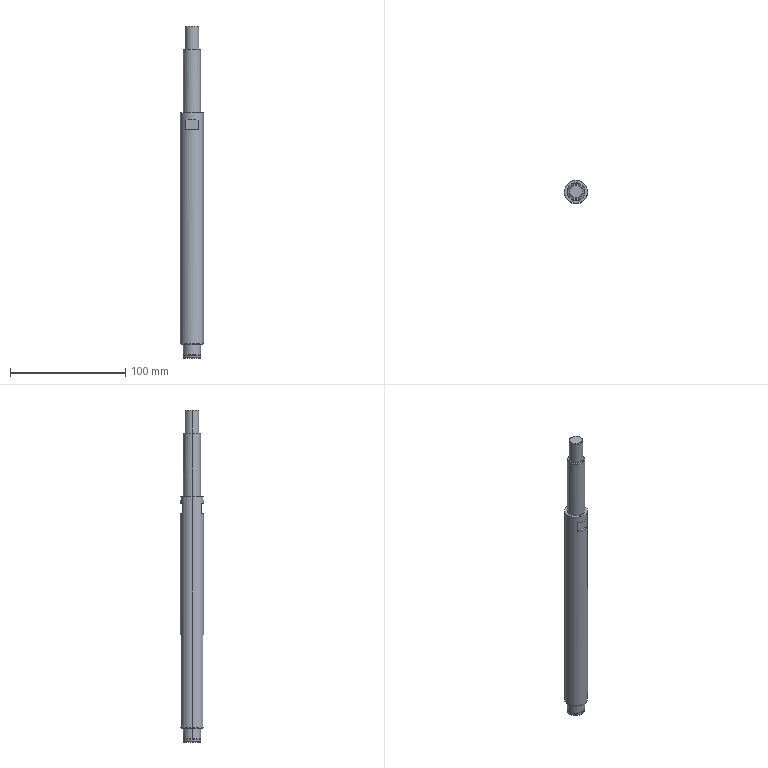Part | SolidWorks | features BaseBody 1 | 1 solid | 37 faces | box 20 x 20 x 287.5 mm | volume 76758 mm3 | plane 13 | cylinder 12 | cone 8 | spline 4 | commonest cylinder face diameters 15 x6 12 x2 14.3 x2 20 x2
STEP:
#1=CARTESIAN_POINT('',(-127.496,1839.044,-21.2));
#2=VERTEX_POINT('',#1);
#3=CARTESIAN_POINT('',(-134.996,1831.544,-21.2));
#4=VERTEX_POINT('',#3);
#5=CARTESIAN_POINT('',(-127.496,1831.544,-21.2));
#6=DIRECTION('',(0.,0.,1.));
#7=DIRECTION('',(0.,-1.,0.));
#8=AXIS2_PLACEMENT_3D('',#5,#6,#7);
#9=CIRCLE('',#8,7.5);
#10=EDGE_CURVE('',#2,#4,#9,.T.);
#11=ORIENTED_EDGE('',*,*,#10,.F.);
#12=CARTESIAN_POINT('',(-127.496,1839.344,-21.5));
#13=VERTEX_POINT('',#12);
#14=CARTESIAN_POINT('',(-127.496,1839.344,-21.2));
#15=DIRECTION('',(1.,0.,0.));
#16=DIRECTION('',(0.,1.,0.));
#17=AXIS2_PLACEMENT_3D('',#14,#15,#16);
#18=CIRCLE('',#17,0.3);
#19=EDGE_CURVE('',#2,#13,#18,.T.);
#20=ORIENTED_EDGE('',*,*,#19,.T.);
#21=CARTESIAN_POINT('',(-127.496,1823.744,-21.5));
#22=VERTEX_POINT('',#21);
#23=CARTESIAN_POINT('',(-127.496,1839.344,-21.5));
#24=CARTESIAN_POINT('',(-143.096,1839.344,-21.5));
#25=CARTESIAN_POINT('',(-143.096,1823.744,-21.5));
#26=CARTESIAN_POINT('',(-127.496,1823.744,-21.5));
#27=(BOUNDED_CURVE()B_SPLINE_CURVE(3,(#23,#24,#25,#26),.UNSPECIFIED.,.F.,.F.)B_SPLINE_CURVE_WITH_KNOTS((4,4),(0.,1.),.UNSPECIFIED.)CURVE()GEOMETRIC_REPRESENTATION_ITEM()RATIONAL_B_SPLINE_CURVE((1.,0.3333,0.3333,1.))REPRESENTATION_ITEM(''));
#28=EDGE_CURVE('',#13,#22,#27,.T.);
#29=ORIENTED_EDGE('',*,*,#28,.T.);
#30=CARTESIAN_POINT('',(-127.496,1824.044,-21.2));
#31=VERTEX_POINT('',#30);
#32=CARTESIAN_POINT('',(-127.496,1823.744,-21.2));
#33=DIRECTION('',(-1.,0.,0.));
#34=DIRECTION('',(0.,-1.,0.));
#35=AXIS2_PLACEMENT_3D('',#32,#33,#34);
#36=CIRCLE('',#35,0.3);
#37=EDGE_CURVE('',#31,#22,#36,.T.);
#38=ORIENTED_EDGE('',*,*,#37,.F.);
#39=CARTESIAN_POINT('',(-127.496,1831.544,-21.2));
#40=DIRECTION('',(0.,0.,1.));
#41=DIRECTION('',(0.,-1.,0.));
#42=AXIS2_PLACEMENT_3D('',#39,#40,#41);
#43=CIRCLE('',#42,7.5);
#44=EDGE_CURVE('',#4,#31,#43,.T.);
#45=ORIENTED_EDGE('',*,*,#44,.F.);
#46=EDGE_LOOP('',(#11,#20,#29,#38,#45));
#47=FACE_OUTER_BOUND('',#46,.T.);
#48=CARTESIAN_POINT('',(-127.496,1824.044,-21.2));
#49=CARTESIAN_POINT('',(-142.496,1824.044,-21.2));
#50=CARTESIAN_POINT('',(-142.496,1839.044,-21.2));
#51=CARTESIAN_POINT('',(-127.496,1839.044,-21.2));
#52=CARTESIAN_POINT('',(-127.496,1824.044,-21.376));
#53=CARTESIAN_POINT('',(-142.496,1824.044,-21.376));
#54=CARTESIAN_POINT('',(-142.496,1839.044,-21.376));
#55=CARTESIAN_POINT('',(-127.496,1839.044,-21.376));
#56=CARTESIAN_POINT('',(-127.496,1823.92,-21.5));
#57=CARTESIAN_POINT('',(-142.744,1823.92,-21.5));
#58=CARTESIAN_POINT('',(-142.744,1839.168,-21.5));
#59=CARTESIAN_POINT('',(-127.496,1839.168,-21.5));
#60=CARTESIAN_POINT('',(-127.496,1823.744,-21.5));
#61=CARTESIAN_POINT('',(-143.096,1823.744,-21.5));
#62=CARTESIAN_POINT('',(-143.096,1839.344,-21.5));
#63=CARTESIAN_POINT('',(-127.496,1839.344,-21.5));
#64=(BOUNDED_SURFACE()B_SPLINE_SURFACE(3,3,((#48,#49,#50,#51),(#52,#53,#54,#55),(#56,#57,#58,#59),(#60,#61,#62,#63)),.UNSPECIFIED.,.F.,.F.,.T.)B_SPLINE_SURFACE_WITH_KNOTS((4,4),(4,4),(0.,1.),(0.,1.),.UNSPECIFIED.)GEOMETRIC_REPRESENTATION_ITEM()RATIONAL_B_SPLINE_SURFACE(((1.,0.3333,0.3333,1.),(0.8047,0.2682,0.2682,0.8047),(0.8047,0.2682,0.2682,0.8047),(1.,0.3333,0.3333,1.)))REPRESENTATION_ITEM('')SURFACE());
#65=ADVANCED_FACE('',(#47),#64,.F.);
#66=CARTESIAN_POINT('',(-127.496,1824.044,-222.3));
#67=VERTEX_POINT('',#66);
#68=CARTESIAN_POINT('',(-134.996,1831.544,-222.3));
#69=VERTEX_POINT('',#68);
#70=CARTESIAN_POINT('',(-127.496,1831.544,-222.3));
#71=DIRECTION('',(0.,0.,-1.));
#72=DIRECTION('',(0.,1.,0.));
#73=AXIS2_PLACEMENT_3D('',#70,#71,#72);
#74=CIRCLE('',#73,7.5);
#75=EDGE_CURVE('',#67,#69,#74,.T.);
#76=ORIENTED_EDGE('',*,*,#75,.F.);
#77=CARTESIAN_POINT('',(-127.496,1823.744,-222.));
#78=VERTEX_POINT('',#77);
#79=CARTESIAN_POINT('',(-127.496,1823.744,-222.3));
#80=DIRECTION('',(1.,0.,0.));
#81=DIRECTION('',(0.,-1.,0.));
#82=AXIS2_PLACEMENT_3D('',#79,#80,#81);
#83=CIRCLE('',#82,0.3);
#84=EDGE_CURVE('',#67,#78,#83,.T.);
#85=ORIENTED_EDGE('',*,*,#84,.T.);
#86=CARTESIAN_POINT('',(-127.496,1839.344,-222.));
#87=VERTEX_POINT('',#86);
#88=CARTESIAN_POINT('',(-127.496,1823.744,-222.));
#89=CARTESIAN_POINT('',(-143.096,1823.744,-222.));
#90=CARTESIAN_POINT('',(-143.096,1839.344,-222.));
#91=CARTESIAN_POINT('',(-127.496,1839.344,-222.));
#92=(BOUNDED_CURVE()B_SPLINE_CURVE(3,(#88,#89,#90,#91),.UNSPECIFIED.,.F.,.F.)B_SPLINE_CURVE_WITH_KNOTS((4,4),(0.,1.),.UNSPECIFIED.)CURVE()GEOMETRIC_REPRESENTATION_ITEM()RATIONAL_B_SPLINE_CURVE((1.,0.3333,0.3333,1.))REPRESENTATION_ITEM(''));
#93=EDGE_CURVE('',#78,#87,#92,.T.);
#94=ORIENTED_EDGE('',*,*,#93,.T.);
#95=CARTESIAN_POINT('',(-127.496,1839.044,-222.3));
#96=VERTEX_POINT('',#95);
#97=CARTESIAN_POINT('',(-127.496,1839.344,-222.3));
#98=DIRECTION('',(-1.,0.,0.));
#99=DIRECTION('',(0.,1.,0.));
#100=AXIS2_PLACEMENT_3D('',#97,#98,#99);
#101=CIRCLE('',#100,0.3);
#102=EDGE_CURVE('',#96,#87,#101,.T.);
#103=ORIENTED_EDGE('',*,*,#102,.F.);
#104=CARTESIAN_POINT('',(-127.496,1831.544,-222.3));
#105=DIRECTION('',(0.,0.,-1.));
#106=DIRECTION('',(0.,1.,0.));
#107=AXIS2_PLACEMENT_3D('',#104,#105,#106);
#108=CIRCLE('',#107,7.5);
#109=EDGE_CURVE('',#69,#96,#108,.T.);
#110=ORIENTED_EDGE('',*,*,#109,.F.);
#111=EDGE_LOOP('',(#76,#85,#94,#103,#110));
#112=FACE_OUTER_BOUND('',#111,.T.);
#113=CARTESIAN_POINT('',(-127.496,1839.044,-222.3));
#114=CARTESIAN_POINT('',(-142.496,1839.044,-222.3));
#115=CARTESIAN_POINT('',(-142.496,1824.044,-222.3));
#116=CARTESIAN_POINT('',(-127.496,1824.044,-222.3));
#117=CARTESIAN_POINT('',(-127.496,1839.044,-222.124));
#118=CARTESIAN_POINT('',(-142.496,1839.044,-222.124));
#119=CARTESIAN_POINT('',(-142.496,1824.044,-222.124));
#120=CARTESIAN_POINT('',(-127.496,1824.044,-222.124));
#121=CARTESIAN_POINT('',(-127.496,1839.168,-222.));
#122=CARTESIAN_POINT('',(-142.744,1839.168,-222.));
#123=CARTESIAN_POINT('',(-142.744,1823.92,-222.));
#124=CARTESIAN_POINT('',(-127.496,1823.92,-222.));
#125=CARTESIAN_POINT('',(-127.496,1839.344,-222.));
#126=CARTESIAN_POINT('',(-143.096,1839.344,-222.));
#127=CARTESIAN_POINT('',(-143.096,1823.744,-222.));
#128=CARTESIAN_POINT('',(-127.496,1823.744,-222.));
#129=(BOUNDED_SURFACE()B_SPLINE_SURFACE(3,3,((#113,#114,#115,#116),(#117,#118,#119,#120),(#121,#122,#123,#124),(#125,#126,#127,#128)),.UNSPECIFIED.,.F.,.F.,.T.)B_SPLINE_SURFACE_WITH_KNOTS((4,4),(4,4),(0.,1.),(0.,1.),.UNSPECIFIED.)GEOMETRIC_REPRESENTATION_ITEM()RATIONAL_B_SPLINE_SURFACE(((1.,0.3333,0.3333,1.),(0.8047,0.2682,0.2682,0.8047),(0.8047,0.2682,0.2682,0.8047),(1.,0.3333,0.3333,1.)))REPRESENTATION_ITEM('')SURFACE());
#130=ADVANCED_FACE('',(#112),#129,.F.);
#131=CARTESIAN_POINT('',(-133.496,1839.544,-27.5));
#132=VERTEX_POINT('',#131);
#133=CARTESIAN_POINT('',(-133.496,1839.544,-36.5));
#134=VERTEX_POINT('',#133);
#135=CARTESIAN_POINT('',(-133.496,1839.544,13.5));
#136=DIRECTION('',(0.,0.,-1.));
#137=VECTOR('',#136,1000.);
#138=LINE('',#135,#137);
#139=EDGE_CURVE('',#132,#134,#138,.T.);
#140=ORIENTED_EDGE('',*,*,#139,.T.);
#141=CARTESIAN_POINT('',(-121.496,1839.544,-36.5));
#142=VERTEX_POINT('',#141);
#143=CARTESIAN_POINT('',(-127.496,1831.544,-36.5));
#144=DIRECTION('',(0.,0.,-1.));
#145=DIRECTION('',(-1.,0.,0.));
#146=AXIS2_PLACEMENT_3D('',#143,#144,#145);
#147=CIRCLE('',#146,10.);
#148=EDGE_CURVE('',#134,#142,#147,.T.);
#149=ORIENTED_EDGE('',*,*,#148,.T.);
#150=CARTESIAN_POINT('',(-121.496,1839.544,-27.5));
#151=VERTEX_POINT('',#150);
#152=CARTESIAN_POINT('',(-121.496,1839.544,13.5));
#153=DIRECTION('',(0.,0.,1.));
#154=VECTOR('',#153,1000.);
#155=LINE('',#152,#154);
#156=EDGE_CURVE('',#142,#151,#155,.T.);
#157=ORIENTED_EDGE('',*,*,#156,.T.);
#158=CARTESIAN_POINT('',(-127.496,1831.544,-27.5));
#159=DIRECTION('',(0.,0.,1.));
#160=DIRECTION('',(-1.,0.,0.));
#161=AXIS2_PLACEMENT_3D('',#158,#159,#160);
#162=CIRCLE('',#161,10.);
#163=EDGE_CURVE('',#151,#132,#162,.T.);
#164=ORIENTED_EDGE('',*,*,#163,.T.);
#165=EDGE_LOOP('',(#140,#149,#157,#164));
#166=FACE_BOUND('',#165,.T.);
#167=CARTESIAN_POINT('',(-137.496,1831.544,-21.5));
#168=VERTEX_POINT('',#167);
#169=CARTESIAN_POINT('',(-117.496,1831.544,-21.5));
#170=VERTEX_POINT('',#169);
#171=CARTESIAN_POINT('',(-127.496,1831.544,-21.5));
#172=DIRECTION('',(0.,0.,-1.));
#173=DIRECTION('',(-1.,0.,0.));
#174=AXIS2_PLACEMENT_3D('',#171,#172,#173);
#175=CIRCLE('',#174,10.);
#176=EDGE_CURVE('',#168,#170,#175,.T.);
#177=ORIENTED_EDGE('',*,*,#176,.T.);
#178=CARTESIAN_POINT('',(-117.496,1831.544,-221.5));
#179=VERTEX_POINT('',#178);
#180=CARTESIAN_POINT('',(-117.496,1831.544,13.5));
#181=DIRECTION('',(0.,0.,-1.));
#182=VECTOR('',#181,1000.);
#183=LINE('',#180,#182);
#184=EDGE_CURVE('',#170,#179,#183,.T.);
#185=ORIENTED_EDGE('',*,*,#184,.T.);
#186=CARTESIAN_POINT('',(-137.496,1831.544,-221.5));
#187=VERTEX_POINT('',#186);
#188=CARTESIAN_POINT('',(-127.496,1831.544,-221.5));
#189=DIRECTION('',(0.,0.,1.));
#190=DIRECTION('',(-1.,0.,0.));
#191=AXIS2_PLACEMENT_3D('',#188,#189,#190);
#192=CIRCLE('',#191,10.);
#193=EDGE_CURVE('',#179,#187,#192,.T.);
#194=ORIENTED_EDGE('',*,*,#193,.T.);
#195=CARTESIAN_POINT('',(-137.496,1831.544,13.5));
#196=DIRECTION('',(0.,0.,-1.));
#197=VECTOR('',#196,1000.);
#198=LINE('',#195,#197);
#199=EDGE_CURVE('',#168,#187,#198,.T.);
#200=ORIENTED_EDGE('',*,*,#199,.F.);
#201=EDGE_LOOP('',(#177,#185,#194,#200));
#202=FACE_OUTER_BOUND('',#201,.T.);
#203=CARTESIAN_POINT('',(-127.496,1831.544,13.5));
#204=DIRECTION('',(0.,0.,-1.));
#205=DIRECTION('',(-1.,0.,0.));
#206=AXIS2_PLACEMENT_3D('',#203,#204,#205);
#207=CYLINDRICAL_SURFACE('',#206,10.);
#208=ADVANCED_FACE('',(#166,#202),#207,.T.);
#209=CARTESIAN_POINT('',(-117.996,1831.544,-222.));
#210=VERTEX_POINT('',#209);
#211=CARTESIAN_POINT('',(-136.996,1831.544,-222.));
#212=VERTEX_POINT('',#211);
#213=CARTESIAN_POINT('',(-127.496,1831.544,-222.));
#214=DIRECTION('',(0.,0.,1.));
#215=DIRECTION('',(1.,0.,0.));
#216=AXIS2_PLACEMENT_3D('',#213,#214,#215);
#217=CIRCLE('',#216,9.5);
#218=EDGE_CURVE('',#210,#212,#217,.T.);
#219=ORIENTED_EDGE('',*,*,#218,.T.);
#220=CARTESIAN_POINT('',(-137.496,1831.544,-221.5));
#221=DIRECTION('',(-0.7071,0.,0.7071));
#222=VECTOR('',#221,1000.);
#223=LINE('',#220,#222);
#224=EDGE_CURVE('',#212,#187,#223,.T.);
#225=ORIENTED_EDGE('',*,*,#224,.T.);
#226=ORIENTED_EDGE('',*,*,#193,.F.);
#227=CARTESIAN_POINT('',(-117.496,1831.544,-221.5));
#228=DIRECTION('',(0.7071,0.,0.7071));
#229=VECTOR('',#228,1000.);
#230=LINE('',#227,#229);
#231=EDGE_CURVE('',#210,#179,#230,.T.);
#232=ORIENTED_EDGE('',*,*,#231,.F.);
#233=EDGE_LOOP('',(#219,#225,#226,#232));
#234=FACE_OUTER_BOUND('',#233,.T.);
#235=CARTESIAN_POINT('',(-127.496,1831.544,-221.5));
#236=DIRECTION('',(0.,0.,1.));
#237=DIRECTION('',(1.,0.,0.));
#238=AXIS2_PLACEMENT_3D('',#235,#236,#237);
#239=CONICAL_SURFACE('',#238,10.,0.7854);
#240=ADVANCED_FACE('',(#234),#239,.T.);
#241=CARTESIAN_POINT('',(-134.996,1831.544,33.));
#242=VERTEX_POINT('',#241);
#243=CARTESIAN_POINT('',(-119.996,1831.544,33.));
#244=VERTEX_POINT('',#243);
#245=CARTESIAN_POINT('',(-127.496,1831.544,33.));
#246=DIRECTION('',(0.,0.,-1.));
#247=DIRECTION('',(-1.,0.,0.));
#248=AXIS2_PLACEMENT_3D('',#245,#246,#247);
#249=CIRCLE('',#248,7.5);
#250=EDGE_CURVE('',#242,#244,#249,.T.);
#251=ORIENTED_EDGE('',*,*,#250,.T.);
#252=CARTESIAN_POINT('',(-119.996,1831.544,-21.2));
#253=VERTEX_POINT('',#252);
#254=CARTESIAN_POINT('',(-119.996,1831.544,-206.5));
#255=DIRECTION('',(0.,0.,-1.));
#256=VECTOR('',#255,1000.);
#257=LINE('',#254,#256);
#258=EDGE_CURVE('',#244,#253,#257,.T.);
#259=ORIENTED_EDGE('',*,*,#258,.T.);
#260=CARTESIAN_POINT('',(-127.496,1831.544,-21.2));
#261=DIRECTION('',(0.,0.,1.));
#262=DIRECTION('',(0.,-1.,0.));
#263=AXIS2_PLACEMENT_3D('',#260,#261,#262);
#264=CIRCLE('',#263,7.5);
#265=EDGE_CURVE('',#253,#2,#264,.T.);
#266=ORIENTED_EDGE('',*,*,#265,.T.);
#267=ORIENTED_EDGE('',*,*,#10,.T.);
#268=CARTESIAN_POINT('',(-134.996,1831.544,-206.5));
#269=DIRECTION('',(0.,0.,-1.));
#270=VECTOR('',#269,1000.);
#271=LINE('',#268,#270);
#272=EDGE_CURVE('',#242,#4,#271,.T.);
#273=ORIENTED_EDGE('',*,*,#272,.F.);
#274=EDGE_LOOP('',(#251,#259,#266,#267,#273));
#275=FACE_OUTER_BOUND('',#274,.T.);
#276=CARTESIAN_POINT('',(-127.496,1831.544,-206.5));
#277=DIRECTION('',(0.,0.,-1.));
#278=DIRECTION('',(-1.,0.,0.));
#279=AXIS2_PLACEMENT_3D('',#276,#277,#278);
#280=CYLINDRICAL_SURFACE('',#279,7.5);
#281=ADVANCED_FACE('',(#275),#280,.T.);
#282=CARTESIAN_POINT('',(-134.496,1831.544,33.5));
#283=VERTEX_POINT('',#282);
#284=CARTESIAN_POINT('',(-120.496,1831.544,33.5));
#285=VERTEX_POINT('',#284);
#286=CARTESIAN_POINT('',(-127.496,1831.544,33.5));
#287=DIRECTION('',(0.,0.,-1.));
#288=DIRECTION('',(-1.,0.,0.));
#289=AXIS2_PLACEMENT_3D('',#286,#287,#288);
#290=CIRCLE('',#289,7.);
#291=EDGE_CURVE('',#283,#285,#290,.T.);
#292=ORIENTED_EDGE('',*,*,#291,.T.);
#293=CARTESIAN_POINT('',(-119.996,1831.544,33.));
#294=DIRECTION('',(0.7071,0.,-0.7071));
#295=VECTOR('',#294,1000.);
#296=LINE('',#293,#295);
#297=EDGE_CURVE('',#285,#244,#296,.T.);
#298=ORIENTED_EDGE('',*,*,#297,.T.);
#299=ORIENTED_EDGE('',*,*,#250,.F.);
#300=CARTESIAN_POINT('',(-134.996,1831.544,33.));
#301=DIRECTION('',(-0.7071,0.,-0.7071));
#302=VECTOR('',#301,1000.);
#303=LINE('',#300,#302);
#304=EDGE_CURVE('',#283,#242,#303,.T.);
#305=ORIENTED_EDGE('',*,*,#304,.F.);
#306=EDGE_LOOP('',(#292,#298,#299,#305));
#307=FACE_OUTER_BOUND('',#306,.T.);
#308=CARTESIAN_POINT('',(-127.496,1831.544,33.));
#309=DIRECTION('',(0.,0.,-1.));
#310=DIRECTION('',(-1.,0.,0.));
#311=AXIS2_PLACEMENT_3D('',#308,#309,#310);
#312=CONICAL_SURFACE('',#311,7.5,0.7854);
#313=ADVANCED_FACE('',(#307),#312,.T.);
#314=ORIENTED_EDGE('',*,*,#109,.T.);
#315=CARTESIAN_POINT('',(-119.996,1831.544,-222.3));
#316=VERTEX_POINT('',#315);
#317=CARTESIAN_POINT('',(-127.496,1831.544,-222.3));
#318=DIRECTION('',(0.,0.,-1.));
#319=DIRECTION('',(0.,1.,0.));
#320=AXIS2_PLACEMENT_3D('',#317,#318,#319);
#321=CIRCLE('',#320,7.5);
#322=EDGE_CURVE('',#96,#316,#321,.T.);
#323=ORIENTED_EDGE('',*,*,#322,.T.);
#324=CARTESIAN_POINT('',(-119.996,1831.544,-231.));
#325=VERTEX_POINT('',#324);
#326=CARTESIAN_POINT('',(-119.996,1831.544,-234.));
#327=DIRECTION('',(0.,0.,-1.));
#328=VECTOR('',#327,1000.);
#329=LINE('',#326,#328);
#330=EDGE_CURVE('',#316,#325,#329,.T.);
#331=ORIENTED_EDGE('',*,*,#330,.T.);
#332=CARTESIAN_POINT('',(-134.996,1831.544,-231.));
#333=VERTEX_POINT('',#332);
#334=CARTESIAN_POINT('',(-127.496,1831.544,-231.));
#335=DIRECTION('',(0.,0.,1.));
#336=DIRECTION('',(-1.,0.,0.));
#337=AXIS2_PLACEMENT_3D('',#334,#335,#336);
#338=CIRCLE('',#337,7.5);
#339=EDGE_CURVE('',#325,#333,#338,.T.);
#340=ORIENTED_EDGE('',*,*,#339,.T.);
#341=CARTESIAN_POINT('',(-134.996,1831.544,-234.));
#342=DIRECTION('',(0.,0.,-1.));
#343=VECTOR('',#342,1000.);
#344=LINE('',#341,#343);
#345=EDGE_CURVE('',#69,#333,#344,.T.);
#346=ORIENTED_EDGE('',*,*,#345,.F.);
#347=EDGE_LOOP('',(#314,#323,#331,#340,#346));
#348=FACE_OUTER_BOUND('',#347,.T.);
#349=CARTESIAN_POINT('',(-127.496,1831.544,-234.));
#350=DIRECTION('',(0.,0.,-1.));
#351=DIRECTION('',(-1.,0.,0.));
#352=AXIS2_PLACEMENT_3D('',#349,#350,#351);
#353=CYLINDRICAL_SURFACE('',#352,7.5);
#354=ADVANCED_FACE('',(#348),#353,.T.);
#355=CARTESIAN_POINT('',(-133.496,1831.544,53.));
#356=VERTEX_POINT('',#355);
#357=CARTESIAN_POINT('',(-121.496,1831.544,53.));
#358=VERTEX_POINT('',#357);
#359=CARTESIAN_POINT('',(-127.496,1831.544,53.));
#360=DIRECTION('',(0.,0.,-1.));
#361=DIRECTION('',(-1.,0.,0.));
#362=AXIS2_PLACEMENT_3D('',#359,#360,#361);
#363=CIRCLE('',#362,6.);
#364=EDGE_CURVE('',#356,#358,#363,.T.);
#365=ORIENTED_EDGE('',*,*,#364,.T.);
#366=CARTESIAN_POINT('',(-121.496,1831.544,33.5));
#367=VERTEX_POINT('',#366);
#368=CARTESIAN_POINT('',(-121.496,1831.544,-206.5));
#369=DIRECTION('',(0.,0.,-1.));
#370=VECTOR('',#369,1000.);
#371=LINE('',#368,#370);
#372=EDGE_CURVE('',#358,#367,#371,.T.);
#373=ORIENTED_EDGE('',*,*,#372,.T.);
#374=CARTESIAN_POINT('',(-133.496,1831.544,33.5));
#375=VERTEX_POINT('',#374);
#376=CARTESIAN_POINT('',(-127.496,1831.544,33.5));
#377=DIRECTION('',(0.,0.,1.));
#378=DIRECTION('',(-1.,0.,0.));
#379=AXIS2_PLACEMENT_3D('',#376,#377,#378);
#380=CIRCLE('',#379,6.);
#381=EDGE_CURVE('',#367,#375,#380,.T.);
#382=ORIENTED_EDGE('',*,*,#381,.T.);
#383=CARTESIAN_POINT('',(-133.496,1831.544,-206.5));
#384=DIRECTION('',(0.,0.,-1.));
#385=VECTOR('',#384,1000.);
#386=LINE('',#383,#385);
#387=EDGE_CURVE('',#356,#375,#386,.T.);
#388=ORIENTED_EDGE('',*,*,#387,.F.);
#389=EDGE_LOOP('',(#365,#373,#382,#388));
#390=FACE_OUTER_BOUND('',#389,.T.);
#391=CARTESIAN_POINT('',(-127.496,1831.544,-206.5));
#392=DIRECTION('',(0.,0.,-1.));
#393=DIRECTION('',(-1.,0.,0.));
#394=AXIS2_PLACEMENT_3D('',#391,#392,#393);
#395=CYLINDRICAL_SURFACE('',#394,6.);
#396=ADVANCED_FACE('',(#390),#395,.T.);
#397=CARTESIAN_POINT('',(-134.646,1831.544,-231.));
#398=VERTEX_POINT('',#397);
#399=CARTESIAN_POINT('',(-120.346,1831.544,-231.));
#400=VERTEX_POINT('',#399);
#401=CARTESIAN_POINT('',(-127.496,1831.544,-231.));
#402=DIRECTION('',(0.,0.,-1.));
#403=DIRECTION('',(-1.,0.,0.));
#404=AXIS2_PLACEMENT_3D('',#401,#402,#403);
#405=CIRCLE('',#404,7.15);
#406=EDGE_CURVE('',#398,#400,#405,.T.);
#407=ORIENTED_EDGE('',*,*,#406,.T.);
#408=CARTESIAN_POINT('',(-120.346,1831.544,-232.15));
#409=VERTEX_POINT('',#408);
#410=CARTESIAN_POINT('',(-120.346,1831.544,-234.));
#411=DIRECTION('',(0.,0.,-1.));
#412=VECTOR('',#411,1000.);
#413=LINE('',#410,#412);
#414=EDGE_CURVE('',#400,#409,#413,.T.);
#415=ORIENTED_EDGE('',*,*,#414,.T.);
#416=CARTESIAN_POINT('',(-134.646,1831.544,-232.15));
#417=VERTEX_POINT('',#416);
#418=CARTESIAN_POINT('',(-127.496,1831.544,-232.15));
#419=DIRECTION('',(0.,0.,1.));
#420=DIRECTION('',(-1.,0.,0.));
#421=AXIS2_PLACEMENT_3D('',#418,#419,#420);
#422=CIRCLE('',#421,7.15);
#423=EDGE_CURVE('',#409,#417,#422,.T.);
#424=ORIENTED_EDGE('',*,*,#423,.T.);
#425=CARTESIAN_POINT('',(-134.646,1831.544,-234.));
#426=DIRECTION('',(0.,0.,-1.));
#427=VECTOR('',#426,1000.);
#428=LINE('',#425,#427);
#429=EDGE_CURVE('',#398,#417,#428,.T.);
#430=ORIENTED_EDGE('',*,*,#429,.F.);
#431=EDGE_LOOP('',(#407,#415,#424,#430));
#432=FACE_OUTER_BOUND('',#431,.T.);
#433=CARTESIAN_POINT('',(-127.496,1831.544,-234.));
#434=DIRECTION('',(0.,0.,-1.));
#435=DIRECTION('',(-1.,0.,0.));
#436=AXIS2_PLACEMENT_3D('',#433,#434,#435);
#437=CYLINDRICAL_SURFACE('',#436,7.15);
#438=ADVANCED_FACE('',(#432),#437,.T.);
#439=CARTESIAN_POINT('',(-132.996,1831.544,53.5));
#440=VERTEX_POINT('',#439);
#441=CARTESIAN_POINT('',(-121.996,1831.544,53.5));
#442=VERTEX_POINT('',#441);
#443=CARTESIAN_POINT('',(-127.496,1831.544,53.5));
#444=DIRECTION('',(0.,0.,-1.));
#445=DIRECTION('',(-1.,0.,0.));
#446=AXIS2_PLACEMENT_3D('',#443,#444,#445);
#447=CIRCLE('',#446,5.5);
#448=EDGE_CURVE('',#440,#442,#447,.T.);
#449=ORIENTED_EDGE('',*,*,#448,.T.);
#450=CARTESIAN_POINT('',(-121.496,1831.544,53.));
#451=DIRECTION('',(0.7071,0.,-0.7071));
#452=VECTOR('',#451,1000.);
#453=LINE('',#450,#452);
#454=EDGE_CURVE('',#442,#358,#453,.T.);
#455=ORIENTED_EDGE('',*,*,#454,.T.);
#456=ORIENTED_EDGE('',*,*,#364,.F.);
#457=CARTESIAN_POINT('',(-133.496,1831.544,53.));
#458=DIRECTION('',(-0.7071,0.,-0.7071));
#459=VECTOR('',#458,1000.);
#460=LINE('',#457,#459);
#461=EDGE_CURVE('',#440,#356,#460,.T.);
#462=ORIENTED_EDGE('',*,*,#461,.F.);
#463=EDGE_LOOP('',(#449,#455,#456,#462));
#464=FACE_OUTER_BOUND('',#463,.T.);
#465=CARTESIAN_POINT('',(-127.496,1831.544,53.));
#466=DIRECTION('',(0.,0.,-1.));
#467=DIRECTION('',(-1.,0.,0.));
#468=AXIS2_PLACEMENT_3D('',#465,#466,#467);
#469=CONICAL_SURFACE('',#468,6.,0.7854);
#470=ADVANCED_FACE('',(#464),#469,.T.);
#471=CARTESIAN_POINT('',(-134.996,1831.544,-232.15));
#472=VERTEX_POINT('',#471);
#473=CARTESIAN_POINT('',(-119.996,1831.544,-232.15));
#474=VERTEX_POINT('',#473);
#475=CARTESIAN_POINT('',(-127.496,1831.544,-232.15));
#476=DIRECTION('',(0.,0.,-1.));
#477=DIRECTION('',(-1.,0.,0.));
#478=AXIS2_PLACEMENT_3D('',#475,#476,#477);
#479=CIRCLE('',#478,7.5);
#480=EDGE_CURVE('',#472,#474,#479,.T.);
#481=ORIENTED_EDGE('',*,*,#480,.T.);
#482=CARTESIAN_POINT('',(-119.996,1831.544,-233.5));
#483=VERTEX_POINT('',#482);
#484=CARTESIAN_POINT('',(-119.996,1831.544,-234.));
#485=DIRECTION('',(0.,0.,-1.));
#486=VECTOR('',#485,1000.);
#487=LINE('',#484,#486);
#488=EDGE_CURVE('',#474,#483,#487,.T.);
#489=ORIENTED_EDGE('',*,*,#488,.T.);
#490=CARTESIAN_POINT('',(-134.996,1831.544,-233.5));
#491=VERTEX_POINT('',#490);
#492=CARTESIAN_POINT('',(-127.496,1831.544,-233.5));
#493=DIRECTION('',(0.,0.,1.));
#494=DIRECTION('',(-1.,0.,0.));
#495=AXIS2_PLACEMENT_3D('',#492,#493,#494);
#496=CIRCLE('',#495,7.5);
#497=EDGE_CURVE('',#483,#491,#496,.T.);
#498=ORIENTED_EDGE('',*,*,#497,.T.);
#499=CARTESIAN_POINT('',(-134.996,1831.544,-234.));
#500=DIRECTION('',(0.,0.,-1.));
#501=VECTOR('',#500,1000.);
#502=LINE('',#499,#501);
#503=EDGE_CURVE('',#472,#491,#502,.T.);
#504=ORIENTED_EDGE('',*,*,#503,.F.);
#505=EDGE_LOOP('',(#481,#489,#498,#504));
#506=FACE_OUTER_BOUND('',#505,.T.);
#507=CARTESIAN_POINT('',(-127.496,1831.544,-234.));
#508=DIRECTION('',(0.,0.,-1.));
#509=DIRECTION('',(-1.,0.,0.));
#510=AXIS2_PLACEMENT_3D('',#507,#508,#509);
#511=CYLINDRICAL_SURFACE('',#510,7.5);
#512=ADVANCED_FACE('',(#506),#511,.T.);
#513=CARTESIAN_POINT('',(-120.496,1831.544,-234.));
#514=VERTEX_POINT('',#513);
#515=CARTESIAN_POINT('',(-134.496,1831.544,-234.));
#516=VERTEX_POINT('',#515);
#517=CARTESIAN_POINT('',(-127.496,1831.544,-234.));
#518=DIRECTION('',(0.,0.,1.));
#519=DIRECTION('',(1.,0.,0.));
#520=AXIS2_PLACEMENT_3D('',#517,#518,#519);
#521=CIRCLE('',#520,7.);
#522=EDGE_CURVE('',#514,#516,#521,.T.);
#523=ORIENTED_EDGE('',*,*,#522,.T.);
#524=CARTESIAN_POINT('',(-134.996,1831.544,-233.5));
#525=DIRECTION('',(-0.7071,0.,0.7071));
#526=VECTOR('',#525,1000.);
#527=LINE('',#524,#526);
#528=EDGE_CURVE('',#516,#491,#527,.T.);
#529=ORIENTED_EDGE('',*,*,#528,.T.);
#530=ORIENTED_EDGE('',*,*,#497,.F.);
#531=CARTESIAN_POINT('',(-119.996,1831.544,-233.5));
#532=DIRECTION('',(0.7071,0.,0.7071));
#533=VECTOR('',#532,1000.);
#534=LINE('',#531,#533);
#535=EDGE_CURVE('',#514,#483,#534,.T.);
#536=ORIENTED_EDGE('',*,*,#535,.F.);
#537=EDGE_LOOP('',(#523,#529,#530,#536));
#538=FACE_OUTER_BOUND('',#537,.T.);
#539=CARTESIAN_POINT('',(-127.496,1831.544,-233.5));
#540=DIRECTION('',(0.,0.,1.));
#541=DIRECTION('',(1.,0.,0.));
#542=AXIS2_PLACEMENT_3D('',#539,#540,#541);
#543=CONICAL_SURFACE('',#542,7.5,0.7854);
#544=ADVANCED_FACE('',(#538),#543,.T.);
#545=ORIENTED_EDGE('',*,*,#184,.F.);
#546=CARTESIAN_POINT('',(-127.496,1831.544,-21.5));
#547=DIRECTION('',(0.,0.,-1.));
#548=DIRECTION('',(-1.,0.,0.));
#549=AXIS2_PLACEMENT_3D('',#546,#547,#548);
#550=CIRCLE('',#549,10.);
#551=EDGE_CURVE('',#170,#168,#550,.T.);
#552=ORIENTED_EDGE('',*,*,#551,.T.);
#553=ORIENTED_EDGE('',*,*,#199,.T.);
#554=CARTESIAN_POINT('',(-127.496,1831.544,-221.5));
#555=DIRECTION('',(0.,0.,1.));
#556=DIRECTION('',(-1.,0.,0.));
#557=AXIS2_PLACEMENT_3D('',#554,#555,#556);
#558=CIRCLE('',#557,10.);
#559=EDGE_CURVE('',#187,#179,#558,.T.);
#560=ORIENTED_EDGE('',*,*,#559,.T.);
#561=EDGE_LOOP('',(#545,#552,#553,#560));
#562=FACE_OUTER_BOUND('',#561,.T.);
#563=CARTESIAN_POINT('',(-121.496,1823.544,-27.5));
#564=VERTEX_POINT('',#563);
#565=CARTESIAN_POINT('',(-121.496,1823.544,-36.5));
#566=VERTEX_POINT('',#565);
#567=CARTESIAN_POINT('',(-121.496,1823.544,13.5));
#568=DIRECTION('',(0.,0.,-1.));
#569=VECTOR('',#568,1000.);
#570=LINE('',#567,#569);
#571=EDGE_CURVE('',#564,#566,#570,.T.);
#572=ORIENTED_EDGE('',*,*,#571,.T.);
#573=CARTESIAN_POINT('',(-133.496,1823.544,-36.5));
#574=VERTEX_POINT('',#573);
#575=CARTESIAN_POINT('',(-127.496,1831.544,-36.5));
#576=DIRECTION('',(0.,0.,-1.));
#577=DIRECTION('',(-1.,0.,0.));
#578=AXIS2_PLACEMENT_3D('',#575,#576,#577);
#579=CIRCLE('',#578,10.);
#580=EDGE_CURVE('',#566,#574,#579,.T.);
#581=ORIENTED_EDGE('',*,*,#580,.T.);
#582=CARTESIAN_POINT('',(-133.496,1823.544,-27.5));
#583=VERTEX_POINT('',#582);
#584=CARTESIAN_POINT('',(-133.496,1823.544,-36.5));
#585=DIRECTION('',(0.,0.,1.));
#586=VECTOR('',#585,1000.);
#587=LINE('',#584,#586);
#588=EDGE_CURVE('',#574,#583,#587,.T.);
#589=ORIENTED_EDGE('',*,*,#588,.T.);
#590=CARTESIAN_POINT('',(-127.496,1831.544,-27.5));
#591=DIRECTION('',(0.,0.,1.));
#592=DIRECTION('',(-1.,0.,0.));
#593=AXIS2_PLACEMENT_3D('',#590,#591,#592);
#594=CIRCLE('',#593,10.);
#595=EDGE_CURVE('',#583,#564,#594,.T.);
#596=ORIENTED_EDGE('',*,*,#595,.T.);
#597=EDGE_LOOP('',(#572,#581,#589,#596));
#598=FACE_BOUND('',#597,.T.);
#599=CARTESIAN_POINT('',(-127.496,1831.544,13.5));
#600=DIRECTION('',(0.,0.,-1.));
#601=DIRECTION('',(-1.,0.,0.));
#602=AXIS2_PLACEMENT_3D('',#599,#600,#601);
#603=CYLINDRICAL_SURFACE('',#602,10.);
#604=ADVANCED_FACE('',(#562,#598),#603,.T.);
#605=CARTESIAN_POINT('',(-127.496,1823.544,-36.5));
#606=DIRECTION('',(-1.,0.,0.));
#607=VECTOR('',#606,1000.);
#608=LINE('',#605,#607);
#609=EDGE_CURVE('',#566,#574,#608,.T.);
#610=ORIENTED_EDGE('',*,*,#609,.T.);
#611=ORIENTED_EDGE('',*,*,#580,.F.);
#612=EDGE_LOOP('',(#610,#611));
#613=FACE_OUTER_BOUND('',#612,.T.);
#614=CARTESIAN_POINT('',(-127.496,1831.544,-36.5));
#615=DIRECTION('',(0.,0.,1.));
#616=DIRECTION('',(1.,0.,0.));
#617=AXIS2_PLACEMENT_3D('',#614,#615,#616);
#618=PLANE('',#617);
#619=ADVANCED_FACE('',(#613),#618,.T.);
#620=ORIENTED_EDGE('',*,*,#609,.F.);
#621=ORIENTED_EDGE('',*,*,#571,.F.);
#622=CARTESIAN_POINT('',(-133.496,1823.544,-27.5));
#623=DIRECTION('',(1.,0.,0.));
#624=VECTOR('',#623,1000.);
#625=LINE('',#622,#624);
#626=EDGE_CURVE('',#583,#564,#625,.T.);
#627=ORIENTED_EDGE('',*,*,#626,.F.);
#628=ORIENTED_EDGE('',*,*,#588,.F.);
#629=EDGE_LOOP('',(#620,#621,#627,#628));
#630=FACE_OUTER_BOUND('',#629,.T.);
#631=CARTESIAN_POINT('',(-133.496,1823.544,-36.5));
#632=DIRECTION('',(0.,1.,0.));
#633=DIRECTION('',(0.,0.,1.));
#634=AXIS2_PLACEMENT_3D('',#631,#632,#633);
#635=PLANE('',#634);
#636=ADVANCED_FACE('',(#630),#635,.F.);
#637=ORIENTED_EDGE('',*,*,#626,.T.);
#638=ORIENTED_EDGE('',*,*,#595,.F.);
#639=EDGE_LOOP('',(#637,#638));
#640=FACE_OUTER_BOUND('',#639,.T.);
#641=CARTESIAN_POINT('',(-127.496,1831.544,-27.5));
#642=DIRECTION('',(0.,0.,1.));
#643=DIRECTION('',(1.,0.,0.));
#644=AXIS2_PLACEMENT_3D('',#641,#642,#643);
#645=PLANE('',#644);
#646=ADVANCED_FACE('',(#640),#645,.F.);
#647=ORIENTED_EDGE('',*,*,#28,.F.);
#648=CARTESIAN_POINT('',(-127.496,1823.744,-21.5));
#649=CARTESIAN_POINT('',(-111.896,1823.744,-21.5));
#650=CARTESIAN_POINT('',(-111.896,1839.344,-21.5));
#651=CARTESIAN_POINT('',(-127.496,1839.344,-21.5));
#652=(BOUNDED_CURVE()B_SPLINE_CURVE(3,(#648,#649,#650,#651),.UNSPECIFIED.,.F.,.F.)B_SPLINE_CURVE_WITH_KNOTS((4,4),(0.,1.),.UNSPECIFIED.)CURVE()GEOMETRIC_REPRESENTATION_ITEM()RATIONAL_B_SPLINE_CURVE((1.,0.3333,0.3333,1.))REPRESENTATION_ITEM(''));
#653=EDGE_CURVE('',#22,#13,#652,.T.);
#654=ORIENTED_EDGE('',*,*,#653,.F.);
#655=EDGE_LOOP('',(#647,#654));
#656=FACE_BOUND('',#655,.T.);
#657=ORIENTED_EDGE('',*,*,#176,.F.);
#658=ORIENTED_EDGE('',*,*,#551,.F.);
#659=EDGE_LOOP('',(#657,#658));
#660=FACE_OUTER_BOUND('',#659,.T.);
#661=CARTESIAN_POINT('',(-134.996,1831.544,-21.5));
#662=DIRECTION('',(0.,0.,-1.));
#663=DIRECTION('',(-1.,0.,0.));
#664=AXIS2_PLACEMENT_3D('',#661,#662,#663);
#665=PLANE('',#664);
#666=ADVANCED_FACE('',(#656,#660),#665,.F.);
#667=CARTESIAN_POINT('',(-127.496,1839.544,-27.5));
#668=DIRECTION('',(1.,0.,0.));
#669=VECTOR('',#668,1000.);
#670=LINE('',#667,#669);
#671=EDGE_CURVE('',#132,#151,#670,.T.);
#672=ORIENTED_EDGE('',*,*,#671,.F.);
#673=ORIENTED_EDGE('',*,*,#163,.F.);
#674=EDGE_LOOP('',(#672,#673));
#675=FACE_OUTER_BOUND('',#674,.T.);
#676=CARTESIAN_POINT('',(-127.496,1831.544,-27.5));
#677=DIRECTION('',(0.,0.,1.));
#678=DIRECTION('',(1.,0.,0.));
#679=AXIS2_PLACEMENT_3D('',#676,#677,#678);
#680=PLANE('',#679);
#681=ADVANCED_FACE('',(#675),#680,.F.);
#682=CARTESIAN_POINT('',(-133.496,1839.544,-36.5));
#683=DIRECTION('',(1.,0.,0.));
#684=VECTOR('',#683,1000.);
#685=LINE('',#682,#684);
#686=EDGE_CURVE('',#134,#142,#685,.T.);
#687=ORIENTED_EDGE('',*,*,#686,.F.);
#688=ORIENTED_EDGE('',*,*,#139,.F.);
#689=ORIENTED_EDGE('',*,*,#671,.T.);
#690=ORIENTED_EDGE('',*,*,#156,.F.);
#691=EDGE_LOOP('',(#687,#688,#689,#690));
#692=FACE_OUTER_BOUND('',#691,.T.);
#693=CARTESIAN_POINT('',(-133.496,1839.544,-36.5));
#694=DIRECTION('',(0.,-1.,0.));
#695=DIRECTION('',(0.,0.,-1.));
#696=AXIS2_PLACEMENT_3D('',#693,#694,#695);
#697=PLANE('',#696);
#698=ADVANCED_FACE('',(#692),#697,.F.);
#699=ORIENTED_EDGE('',*,*,#148,.F.);
#700=ORIENTED_EDGE('',*,*,#686,.T.);
#701=EDGE_LOOP('',(#699,#700));
#702=FACE_OUTER_BOUND('',#701,.T.);
#703=CARTESIAN_POINT('',(-127.496,1831.544,-36.5));
#704=DIRECTION('',(0.,0.,1.));
#705=DIRECTION('',(1.,0.,0.));
#706=AXIS2_PLACEMENT_3D('',#703,#704,#705);
#707=PLANE('',#706);
#708=ADVANCED_FACE('',(#702),#707,.T.);
#709=ORIENTED_EDGE('',*,*,#224,.F.);
#710=CARTESIAN_POINT('',(-127.496,1831.544,-222.));
#711=DIRECTION('',(0.,0.,1.));
#712=DIRECTION('',(1.,0.,0.));
#713=AXIS2_PLACEMENT_3D('',#710,#711,#712);
#714=CIRCLE('',#713,9.5);
#715=EDGE_CURVE('',#212,#210,#714,.T.);
#716=ORIENTED_EDGE('',*,*,#715,.T.);
#717=ORIENTED_EDGE('',*,*,#231,.T.);
#718=ORIENTED_EDGE('',*,*,#559,.F.);
#719=EDGE_LOOP('',(#709,#716,#717,#718));
#720=FACE_OUTER_BOUND('',#719,.T.);
#721=CARTESIAN_POINT('',(-127.496,1831.544,-221.5));
#722=DIRECTION('',(0.,0.,1.));
#723=DIRECTION('',(1.,0.,0.));
#724=AXIS2_PLACEMENT_3D('',#721,#722,#723);
#725=CONICAL_SURFACE('',#724,10.,0.7854);
#726=ADVANCED_FACE('',(#720),#725,.T.);
#727=ORIENTED_EDGE('',*,*,#19,.F.);
#728=ORIENTED_EDGE('',*,*,#265,.F.);
#729=CARTESIAN_POINT('',(-127.496,1831.544,-21.2));
#730=DIRECTION('',(0.,0.,1.));
#731=DIRECTION('',(0.,-1.,0.));
#732=AXIS2_PLACEMENT_3D('',#729,#730,#731);
#733=CIRCLE('',#732,7.5);
#734=EDGE_CURVE('',#31,#253,#733,.T.);
#735=ORIENTED_EDGE('',*,*,#734,.F.);
#736=ORIENTED_EDGE('',*,*,#37,.T.);
#737=ORIENTED_EDGE('',*,*,#653,.T.);
#738=EDGE_LOOP('',(#727,#728,#735,#736,#737));
#739=FACE_OUTER_BOUND('',#738,.T.);
#740=CARTESIAN_POINT('',(-127.496,1839.044,-21.2));
#741=CARTESIAN_POINT('',(-112.496,1839.044,-21.2));
#742=CARTESIAN_POINT('',(-112.496,1824.044,-21.2));
#743=CARTESIAN_POINT('',(-127.496,1824.044,-21.2));
#744=CARTESIAN_POINT('',(-127.496,1839.044,-21.376));
#745=CARTESIAN_POINT('',(-112.496,1839.044,-21.376));
#746=CARTESIAN_POINT('',(-112.496,1824.044,-21.376));
#747=CARTESIAN_POINT('',(-127.496,1824.044,-21.376));
#748=CARTESIAN_POINT('',(-127.496,1839.168,-21.5));
#749=CARTESIAN_POINT('',(-112.247,1839.168,-21.5));
#750=CARTESIAN_POINT('',(-112.247,1823.92,-21.5));
#751=CARTESIAN_POINT('',(-127.496,1823.92,-21.5));
#752=CARTESIAN_POINT('',(-127.496,1839.344,-21.5));
#753=CARTESIAN_POINT('',(-111.896,1839.344,-21.5));
#754=CARTESIAN_POINT('',(-111.896,1823.744,-21.5));
#755=CARTESIAN_POINT('',(-127.496,1823.744,-21.5));
#756=(BOUNDED_SURFACE()B_SPLINE_SURFACE(3,3,((#740,#741,#742,#743),(#744,#745,#746,#747),(#748,#749,#750,#751),(#752,#753,#754,#755)),.UNSPECIFIED.,.F.,.F.,.T.)B_SPLINE_SURFACE_WITH_KNOTS((4,4),(4,4),(0.,1.),(0.,1.),.UNSPECIFIED.)GEOMETRIC_REPRESENTATION_ITEM()RATIONAL_B_SPLINE_SURFACE(((1.,0.3333,0.3333,1.),(0.8047,0.2682,0.2682,0.8047),(0.8047,0.2682,0.2682,0.8047),(1.,0.3333,0.3333,1.)))REPRESENTATION_ITEM('')SURFACE());
#757=ADVANCED_FACE('',(#739),#756,.F.);
#758=ORIENTED_EDGE('',*,*,#93,.F.);
#759=CARTESIAN_POINT('',(-127.496,1839.344,-222.));
#760=CARTESIAN_POINT('',(-111.896,1839.344,-222.));
#761=CARTESIAN_POINT('',(-111.896,1823.744,-222.));
#762=CARTESIAN_POINT('',(-127.496,1823.744,-222.));
#763=(BOUNDED_CURVE()B_SPLINE_CURVE(3,(#759,#760,#761,#762),.UNSPECIFIED.,.F.,.F.)B_SPLINE_CURVE_WITH_KNOTS((4,4),(0.,1.),.UNSPECIFIED.)CURVE()GEOMETRIC_REPRESENTATION_ITEM()RATIONAL_B_SPLINE_CURVE((1.,0.3333,0.3333,1.))REPRESENTATION_ITEM(''));
#764=EDGE_CURVE('',#87,#78,#763,.T.);
#765=ORIENTED_EDGE('',*,*,#764,.F.);
#766=EDGE_LOOP('',(#758,#765));
#767=FACE_BOUND('',#766,.T.);
#768=ORIENTED_EDGE('',*,*,#218,.F.);
#769=ORIENTED_EDGE('',*,*,#715,.F.);
#770=EDGE_LOOP('',(#768,#769));
#771=FACE_OUTER_BOUND('',#770,.T.);
#772=CARTESIAN_POINT('',(-137.496,1831.544,-222.));
#773=DIRECTION('',(0.,0.,1.));
#774=DIRECTION('',(1.,0.,0.));
#775=AXIS2_PLACEMENT_3D('',#772,#773,#774);
#776=PLANE('',#775);
#777=ADVANCED_FACE('',(#767,#771),#776,.F.);
#778=ORIENTED_EDGE('',*,*,#84,.F.);
#779=CARTESIAN_POINT('',(-127.496,1831.544,-222.3));
#780=DIRECTION('',(0.,0.,-1.));
#781=DIRECTION('',(0.,1.,0.));
#782=AXIS2_PLACEMENT_3D('',#779,#780,#781);
#783=CIRCLE('',#782,7.5);
#784=EDGE_CURVE('',#316,#67,#783,.T.);
#785=ORIENTED_EDGE('',*,*,#784,.F.);
#786=ORIENTED_EDGE('',*,*,#322,.F.);
#787=ORIENTED_EDGE('',*,*,#102,.T.);
#788=ORIENTED_EDGE('',*,*,#764,.T.);
#789=EDGE_LOOP('',(#778,#785,#786,#787,#788));
#790=FACE_OUTER_BOUND('',#789,.T.);
#791=CARTESIAN_POINT('',(-127.496,1824.044,-222.3));
#792=CARTESIAN_POINT('',(-112.496,1824.044,-222.3));
#793=CARTESIAN_POINT('',(-112.496,1839.044,-222.3));
#794=CARTESIAN_POINT('',(-127.496,1839.044,-222.3));
#795=CARTESIAN_POINT('',(-127.496,1824.044,-222.124));
#796=CARTESIAN_POINT('',(-112.496,1824.044,-222.124));
#797=CARTESIAN_POINT('',(-112.496,1839.044,-222.124));
#798=CARTESIAN_POINT('',(-127.496,1839.044,-222.124));
#799=CARTESIAN_POINT('',(-127.496,1823.92,-222.));
#800=CARTESIAN_POINT('',(-112.247,1823.92,-222.));
#801=CARTESIAN_POINT('',(-112.247,1839.168,-222.));
#802=CARTESIAN_POINT('',(-127.496,1839.168,-222.));
#803=CARTESIAN_POINT('',(-127.496,1823.744,-222.));
#804=CARTESIAN_POINT('',(-111.896,1823.744,-222.));
#805=CARTESIAN_POINT('',(-111.896,1839.344,-222.));
#806=CARTESIAN_POINT('',(-127.496,1839.344,-222.));
#807=(BOUNDED_SURFACE()B_SPLINE_SURFACE(3,3,((#791,#792,#793,#794),(#795,#796,#797,#798),(#799,#800,#801,#802),(#803,#804,#805,#806)),.UNSPECIFIED.,.F.,.F.,.T.)B_SPLINE_SURFACE_WITH_KNOTS((4,4),(4,4),(0.,1.),(0.,1.),.UNSPECIFIED.)GEOMETRIC_REPRESENTATION_ITEM()RATIONAL_B_SPLINE_SURFACE(((1.,0.3333,0.3333,1.),(0.8047,0.2682,0.2682,0.8047),(0.8047,0.2682,0.2682,0.8047),(1.,0.3333,0.3333,1.)))REPRESENTATION_ITEM('')SURFACE());
#808=ADVANCED_FACE('',(#790),#807,.F.);
#809=ORIENTED_EDGE('',*,*,#258,.F.);
#810=CARTESIAN_POINT('',(-127.496,1831.544,33.));
#811=DIRECTION('',(0.,0.,-1.));
#812=DIRECTION('',(-1.,0.,0.));
#813=AXIS2_PLACEMENT_3D('',#810,#811,#812);
#814=CIRCLE('',#813,7.5);
#815=EDGE_CURVE('',#244,#242,#814,.T.);
#816=ORIENTED_EDGE('',*,*,#815,.T.);
#817=ORIENTED_EDGE('',*,*,#272,.T.);
#818=ORIENTED_EDGE('',*,*,#44,.T.);
#819=ORIENTED_EDGE('',*,*,#734,.T.);
#820=EDGE_LOOP('',(#809,#816,#817,#818,#819));
#821=FACE_OUTER_BOUND('',#820,.T.);
#822=CARTESIAN_POINT('',(-127.496,1831.544,-206.5));
#823=DIRECTION('',(0.,0.,-1.));
#824=DIRECTION('',(-1.,0.,0.));
#825=AXIS2_PLACEMENT_3D('',#822,#823,#824);
#826=CYLINDRICAL_SURFACE('',#825,7.5);
#827=ADVANCED_FACE('',(#821),#826,.T.);
#828=ORIENTED_EDGE('',*,*,#297,.F.);
#829=CARTESIAN_POINT('',(-127.496,1831.544,33.5));
#830=DIRECTION('',(0.,0.,-1.));
#831=DIRECTION('',(-1.,0.,0.));
#832=AXIS2_PLACEMENT_3D('',#829,#830,#831);
#833=CIRCLE('',#832,7.);
#834=EDGE_CURVE('',#285,#283,#833,.T.);
#835=ORIENTED_EDGE('',*,*,#834,.T.);
#836=ORIENTED_EDGE('',*,*,#304,.T.);
#837=ORIENTED_EDGE('',*,*,#815,.F.);
#838=EDGE_LOOP('',(#828,#835,#836,#837));
#839=FACE_OUTER_BOUND('',#838,.T.);
#840=CARTESIAN_POINT('',(-127.496,1831.544,33.));
#841=DIRECTION('',(0.,0.,-1.));
#842=DIRECTION('',(-1.,0.,0.));
#843=AXIS2_PLACEMENT_3D('',#840,#841,#842);
#844=CONICAL_SURFACE('',#843,7.5,0.7854);
#845=ADVANCED_FACE('',(#839),#844,.T.);
#846=ORIENTED_EDGE('',*,*,#330,.F.);
#847=ORIENTED_EDGE('',*,*,#784,.T.);
#848=ORIENTED_EDGE('',*,*,#75,.T.);
#849=ORIENTED_EDGE('',*,*,#345,.T.);
#850=CARTESIAN_POINT('',(-127.496,1831.544,-231.));
#851=DIRECTION('',(0.,0.,1.));
#852=DIRECTION('',(-1.,0.,0.));
#853=AXIS2_PLACEMENT_3D('',#850,#851,#852);
#854=CIRCLE('',#853,7.5);
#855=EDGE_CURVE('',#333,#325,#854,.T.);
#856=ORIENTED_EDGE('',*,*,#855,.T.);
#857=EDGE_LOOP('',(#846,#847,#848,#849,#856));
#858=FACE_OUTER_BOUND('',#857,.T.);
#859=CARTESIAN_POINT('',(-127.496,1831.544,-234.));
#860=DIRECTION('',(0.,0.,-1.));
#861=DIRECTION('',(-1.,0.,0.));
#862=AXIS2_PLACEMENT_3D('',#859,#860,#861);
#863=CYLINDRICAL_SURFACE('',#862,7.5);
#864=ADVANCED_FACE('',(#858),#863,.T.);
#865=CARTESIAN_POINT('',(-127.496,1831.544,33.5));
#866=DIRECTION('',(0.,0.,1.));
#867=DIRECTION('',(-1.,0.,0.));
#868=AXIS2_PLACEMENT_3D('',#865,#866,#867);
#869=CIRCLE('',#868,6.);
#870=EDGE_CURVE('',#375,#367,#869,.T.);
#871=ORIENTED_EDGE('',*,*,#870,.F.);
#872=ORIENTED_EDGE('',*,*,#381,.F.);
#873=EDGE_LOOP('',(#871,#872));
#874=FACE_BOUND('',#873,.T.);
#875=ORIENTED_EDGE('',*,*,#291,.F.);
#876=ORIENTED_EDGE('',*,*,#834,.F.);
#877=EDGE_LOOP('',(#875,#876));
#878=FACE_OUTER_BOUND('',#877,.T.);
#879=CARTESIAN_POINT('',(-133.496,1831.544,33.5));
#880=DIRECTION('',(0.,0.,-1.));
#881=DIRECTION('',(-1.,0.,0.));
#882=AXIS2_PLACEMENT_3D('',#879,#880,#881);
#883=PLANE('',#882);
#884=ADVANCED_FACE('',(#874,#878),#883,.F.);
#885=ORIENTED_EDGE('',*,*,#406,.F.);
#886=CARTESIAN_POINT('',(-127.496,1831.544,-231.));
#887=DIRECTION('',(0.,0.,-1.));
#888=DIRECTION('',(-1.,0.,0.));
#889=AXIS2_PLACEMENT_3D('',#886,#887,#888);
#890=CIRCLE('',#889,7.15);
#891=EDGE_CURVE('',#400,#398,#890,.T.);
#892=ORIENTED_EDGE('',*,*,#891,.F.);
#893=EDGE_LOOP('',(#885,#892));
#894=FACE_BOUND('',#893,.T.);
#895=ORIENTED_EDGE('',*,*,#855,.F.);
#896=ORIENTED_EDGE('',*,*,#339,.F.);
#897=EDGE_LOOP('',(#895,#896));
#898=FACE_OUTER_BOUND('',#897,.T.);
#899=CARTESIAN_POINT('',(-134.996,1831.544,-231.));
#900=DIRECTION('',(0.,0.,1.));
#901=DIRECTION('',(1.,0.,0.));
#902=AXIS2_PLACEMENT_3D('',#899,#900,#901);
#903=PLANE('',#902);
#904=ADVANCED_FACE('',(#894,#898),#903,.F.);
#905=ORIENTED_EDGE('',*,*,#372,.F.);
#906=CARTESIAN_POINT('',(-127.496,1831.544,53.));
#907=DIRECTION('',(0.,0.,-1.));
#908=DIRECTION('',(-1.,0.,0.));
#909=AXIS2_PLACEMENT_3D('',#906,#907,#908);
#910=CIRCLE('',#909,6.);
#911=EDGE_CURVE('',#358,#356,#910,.T.);
#912=ORIENTED_EDGE('',*,*,#911,.T.);
#913=ORIENTED_EDGE('',*,*,#387,.T.);
#914=ORIENTED_EDGE('',*,*,#870,.T.);
#915=EDGE_LOOP('',(#905,#912,#913,#914));
#916=FACE_OUTER_BOUND('',#915,.T.);
#917=CARTESIAN_POINT('',(-127.496,1831.544,-206.5));
#918=DIRECTION('',(0.,0.,-1.));
#919=DIRECTION('',(-1.,0.,0.));
#920=AXIS2_PLACEMENT_3D('',#917,#918,#919);
#921=CYLINDRICAL_SURFACE('',#920,6.);
#922=ADVANCED_FACE('',(#916),#921,.T.);
#923=ORIENTED_EDGE('',*,*,#414,.F.);
#924=ORIENTED_EDGE('',*,*,#891,.T.);
#925=ORIENTED_EDGE('',*,*,#429,.T.);
#926=CARTESIAN_POINT('',(-127.496,1831.544,-232.15));
#927=DIRECTION('',(0.,0.,1.));
#928=DIRECTION('',(-1.,0.,0.));
#929=AXIS2_PLACEMENT_3D('',#926,#927,#928);
#930=CIRCLE('',#929,7.15);
#931=EDGE_CURVE('',#417,#409,#930,.T.);
#932=ORIENTED_EDGE('',*,*,#931,.T.);
#933=EDGE_LOOP('',(#923,#924,#925,#932));
#934=FACE_OUTER_BOUND('',#933,.T.);
#935=CARTESIAN_POINT('',(-127.496,1831.544,-234.));
#936=DIRECTION('',(0.,0.,-1.));
#937=DIRECTION('',(-1.,0.,0.));
#938=AXIS2_PLACEMENT_3D('',#935,#936,#937);
#939=CYLINDRICAL_SURFACE('',#938,7.15);
#940=ADVANCED_FACE('',(#934),#939,.T.);
#941=ORIENTED_EDGE('',*,*,#454,.F.);
#942=CARTESIAN_POINT('',(-127.496,1831.544,53.5));
#943=DIRECTION('',(0.,0.,-1.));
#944=DIRECTION('',(-1.,0.,0.));
#945=AXIS2_PLACEMENT_3D('',#942,#943,#944);
#946=CIRCLE('',#945,5.5);
#947=EDGE_CURVE('',#442,#440,#946,.T.);
#948=ORIENTED_EDGE('',*,*,#947,.T.);
#949=ORIENTED_EDGE('',*,*,#461,.T.);
#950=ORIENTED_EDGE('',*,*,#911,.F.);
#951=EDGE_LOOP('',(#941,#948,#949,#950));
#952=FACE_OUTER_BOUND('',#951,.T.);
#953=CARTESIAN_POINT('',(-127.496,1831.544,53.));
#954=DIRECTION('',(0.,0.,-1.));
#955=DIRECTION('',(-1.,0.,0.));
#956=AXIS2_PLACEMENT_3D('',#953,#954,#955);
#957=CONICAL_SURFACE('',#956,6.,0.7854);
#958=ADVANCED_FACE('',(#952),#957,.T.);
#959=ORIENTED_EDGE('',*,*,#931,.F.);
#960=ORIENTED_EDGE('',*,*,#423,.F.);
#961=EDGE_LOOP('',(#959,#960));
#962=FACE_BOUND('',#961,.T.);
#963=ORIENTED_EDGE('',*,*,#480,.F.);
#964=CARTESIAN_POINT('',(-127.496,1831.544,-232.15));
#965=DIRECTION('',(0.,0.,-1.));
#966=DIRECTION('',(-1.,0.,0.));
#967=AXIS2_PLACEMENT_3D('',#964,#965,#966);
#968=CIRCLE('',#967,7.5);
#969=EDGE_CURVE('',#474,#472,#968,.T.);
#970=ORIENTED_EDGE('',*,*,#969,.F.);
#971=EDGE_LOOP('',(#963,#970));
#972=FACE_OUTER_BOUND('',#971,.T.);
#973=CARTESIAN_POINT('',(-134.646,1831.544,-232.15));
#974=DIRECTION('',(0.,0.,-1.));
#975=DIRECTION('',(-1.,0.,0.));
#976=AXIS2_PLACEMENT_3D('',#973,#974,#975);
#977=PLANE('',#976);
#978=ADVANCED_FACE('',(#962,#972),#977,.F.);
#979=ORIENTED_EDGE('',*,*,#448,.F.);
#980=ORIENTED_EDGE('',*,*,#947,.F.);
#981=EDGE_LOOP('',(#979,#980));
#982=FACE_OUTER_BOUND('',#981,.T.);
#983=CARTESIAN_POINT('',(-127.496,1831.544,53.5));
#984=DIRECTION('',(0.,0.,-1.));
#985=DIRECTION('',(-1.,0.,0.));
#986=AXIS2_PLACEMENT_3D('',#983,#984,#985);
#987=PLANE('',#986);
#988=ADVANCED_FACE('',(#982),#987,.F.);
#989=ORIENTED_EDGE('',*,*,#488,.F.);
#990=ORIENTED_EDGE('',*,*,#969,.T.);
#991=ORIENTED_EDGE('',*,*,#503,.T.);
#992=CARTESIAN_POINT('',(-127.496,1831.544,-233.5));
#993=DIRECTION('',(0.,0.,1.));
#994=DIRECTION('',(-1.,0.,0.));
#995=AXIS2_PLACEMENT_3D('',#992,#993,#994);
#996=CIRCLE('',#995,7.5);
#997=EDGE_CURVE('',#491,#483,#996,.T.);
#998=ORIENTED_EDGE('',*,*,#997,.T.);
#999=EDGE_LOOP('',(#989,#990,#991,#998));
#1000=FACE_OUTER_BOUND('',#999,.T.);
#1001=CARTESIAN_POINT('',(-127.496,1831.544,-234.));
#1002=DIRECTION('',(0.,0.,-1.));
#1003=DIRECTION('',(-1.,0.,0.));
#1004=AXIS2_PLACEMENT_3D('',#1001,#1002,#1003);
#1005=CYLINDRICAL_SURFACE('',#1004,7.5);
#1006=ADVANCED_FACE('',(#1000),#1005,.T.);
#1007=ORIENTED_EDGE('',*,*,#528,.F.);
#1008=CARTESIAN_POINT('',(-127.496,1831.544,-234.));
#1009=DIRECTION('',(0.,0.,1.));
#1010=DIRECTION('',(1.,0.,0.));
#1011=AXIS2_PLACEMENT_3D('',#1008,#1009,#1010);
#1012=CIRCLE('',#1011,7.);
#1013=EDGE_CURVE('',#516,#514,#1012,.T.);
#1014=ORIENTED_EDGE('',*,*,#1013,.T.);
#1015=ORIENTED_EDGE('',*,*,#535,.T.);
#1016=ORIENTED_EDGE('',*,*,#997,.F.);
#1017=EDGE_LOOP('',(#1007,#1014,#1015,#1016));
#1018=FACE_OUTER_BOUND('',#1017,.T.);
#1019=CARTESIAN_POINT('',(-127.496,1831.544,-233.5));
#1020=DIRECTION('',(0.,0.,1.));
#1021=DIRECTION('',(1.,0.,0.));
#1022=AXIS2_PLACEMENT_3D('',#1019,#1020,#1021);
#1023=CONICAL_SURFACE('',#1022,7.5,0.7854);
#1024=ADVANCED_FACE('',(#1018),#1023,.T.);
#1025=ORIENTED_EDGE('',*,*,#522,.F.);
#1026=ORIENTED_EDGE('',*,*,#1013,.F.);
#1027=EDGE_LOOP('',(#1025,#1026));
#1028=FACE_OUTER_BOUND('',#1027,.T.);
#1029=CARTESIAN_POINT('',(-134.996,1831.544,-234.));
#1030=DIRECTION('',(0.,0.,1.));
#1031=DIRECTION('',(1.,0.,0.));
#1032=AXIS2_PLACEMENT_3D('',#1029,#1030,#1031);
#1033=PLANE('',#1032);
#1034=ADVANCED_FACE('',(#1028),#1033,.F.);
#1035=CLOSED_SHELL('',(#65,#130,#208,#240,#281,#313,#354,#396,#438,#470,#512,#544,#604,#619,#636,#646,#666,#681,#698,#708,#726,#757,#777,#808,#827,#845,#864,#884,#904,#922,#940,#958,#978,#988,#1006,#1024,#1034));
#1036=MANIFOLD_SOLID_BREP('',#1035);
#1037=CARTESIAN_POINT('',(0.,0.,0.));
#1038=DIRECTION('',(0.,0.,1.));
#1039=DIRECTION('',(1.,0.,0.));
#1040=AXIS2_PLACEMENT_3D('',#1037,#1038,#1039);
#1041=(LENGTH_UNIT()NAMED_UNIT(*)SI_UNIT(.MILLI.,.METRE.));
#1042=UNCERTAINTY_MEASURE_WITH_UNIT(LENGTH_MEASURE(0.00001),#1041,'','');
#1043=(NAMED_UNIT(*)PLANE_ANGLE_UNIT()SI_UNIT($,.RADIAN.));
#1044=(NAMED_UNIT(*)SI_UNIT($,.STERADIAN.)SOLID_ANGLE_UNIT());
#1045=(GEOMETRIC_REPRESENTATION_CONTEXT(3)GLOBAL_UNCERTAINTY_ASSIGNED_CONTEXT((#1042))GLOBAL_UNIT_ASSIGNED_CONTEXT((#1041,#1043,#1044))REPRESENTATION_CONTEXT('',''));
#1046=ADVANCED_BREP_SHAPE_REPRESENTATION('',(#1036,#1040),#1045);